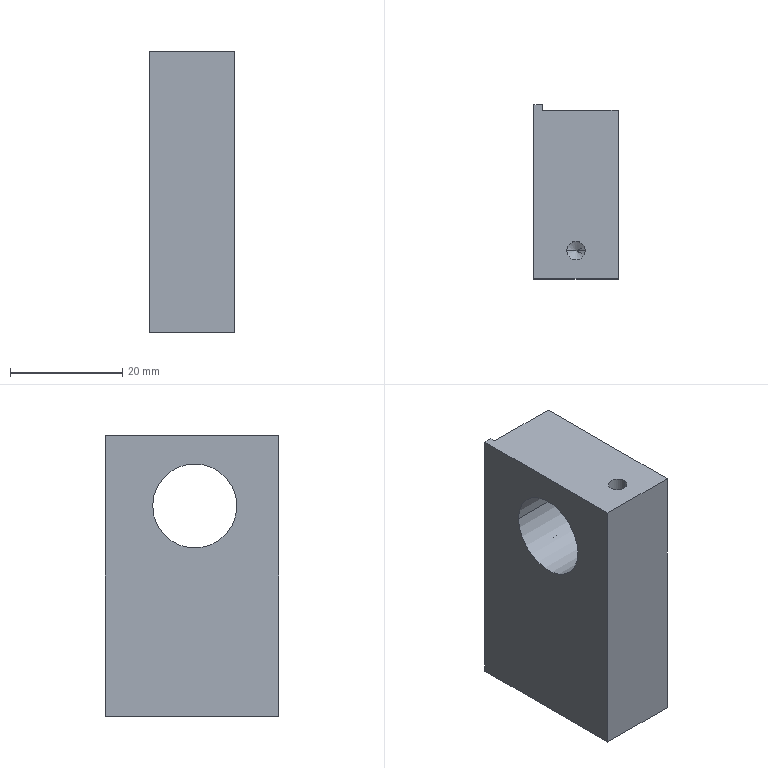Part | STEP file | 11-FG-B01011 | 1 solid | 34 faces | box 15 x 31 x 50 mm | volume 19389 mm3 | cylinder 14 | cone 12 | plane 8 | commonest cylinder face diameters 3.3 x12 15 x2
STEP:
#1=CARTESIAN_POINT('',(5.85,5.,39.9));
#2=VERTEX_POINT('',#1);
#3=CARTESIAN_POINT('',(9.15,5.,39.9));
#4=VERTEX_POINT('',#3);
#5=CARTESIAN_POINT('',(7.5,5.,39.9));
#6=DIRECTION('',(0.,0.,1.));
#7=DIRECTION('',(1.,0.,0.));
#8=AXIS2_PLACEMENT_3D('',#5,#6,#7);
#9=CIRCLE('',#8,1.65);
#10=EDGE_CURVE('',#2,#4,#9,.T.);
#11=ORIENTED_EDGE('',*,*,#10,.F.);
#12=CARTESIAN_POINT('',(5.85,5.,50.));
#13=VERTEX_POINT('',#12);
#14=CARTESIAN_POINT('',(5.85,5.,50.));
#15=DIRECTION('',(0.,0.,1.));
#16=VECTOR('',#15,1000.);
#17=LINE('',#14,#16);
#18=EDGE_CURVE('',#2,#13,#17,.T.);
#19=ORIENTED_EDGE('',*,*,#18,.T.);
#20=CARTESIAN_POINT('',(9.15,5.,50.));
#21=VERTEX_POINT('',#20);
#22=CARTESIAN_POINT('',(7.5,5.,50.));
#23=DIRECTION('',(0.,0.,1.));
#24=DIRECTION('',(1.,0.,0.));
#25=AXIS2_PLACEMENT_3D('',#22,#23,#24);
#26=CIRCLE('',#25,1.65);
#27=EDGE_CURVE('',#13,#21,#26,.T.);
#28=ORIENTED_EDGE('',*,*,#27,.T.);
#29=CARTESIAN_POINT('',(9.15,5.,50.));
#30=DIRECTION('',(0.,0.,1.));
#31=VECTOR('',#30,1000.);
#32=LINE('',#29,#31);
#33=EDGE_CURVE('',#4,#21,#32,.T.);
#34=ORIENTED_EDGE('',*,*,#33,.F.);
#35=EDGE_LOOP('',(#11,#19,#28,#34));
#36=FACE_OUTER_BOUND('',#35,.T.);
#37=CARTESIAN_POINT('',(7.5,5.,50.));
#38=DIRECTION('',(0.,0.,1.));
#39=DIRECTION('',(1.,0.,0.));
#40=AXIS2_PLACEMENT_3D('',#37,#38,#39);
#41=CYLINDRICAL_SURFACE('',#40,1.65);
#42=ADVANCED_FACE('',(#36),#41,.F.);
#43=CARTESIAN_POINT('',(7.5,5.,38.909));
#44=VERTEX_POINT('',#43);
#45=CARTESIAN_POINT('',(9.15,5.,39.9));
#46=DIRECTION('',(0.8572,0.,0.515));
#47=VECTOR('',#46,1000.);
#48=LINE('',#45,#47);
#49=EDGE_CURVE('',#44,#4,#48,.T.);
#50=ORIENTED_EDGE('',*,*,#49,.F.);
#51=CARTESIAN_POINT('',(5.85,5.,39.9));
#52=DIRECTION('',(-0.8572,0.,0.515));
#53=VECTOR('',#52,1000.);
#54=LINE('',#51,#53);
#55=EDGE_CURVE('',#44,#2,#54,.T.);
#56=ORIENTED_EDGE('',*,*,#55,.T.);
#57=ORIENTED_EDGE('',*,*,#10,.T.);
#58=EDGE_LOOP('',(#50,#56,#57));
#59=FACE_OUTER_BOUND('',#58,.T.);
#60=CARTESIAN_POINT('',(7.5,5.,39.9));
#61=DIRECTION('',(0.,0.,1.));
#62=DIRECTION('',(1.,0.,0.));
#63=AXIS2_PLACEMENT_3D('',#60,#61,#62);
#64=CONICAL_SURFACE('',#63,1.65,1.03);
#65=ADVANCED_FACE('',(#59),#64,.F.);
#66=CARTESIAN_POINT('',(6.5,19.9,43.35));
#67=VERTEX_POINT('',#66);
#68=CARTESIAN_POINT('',(6.5,19.9,46.65));
#69=VERTEX_POINT('',#68);
#70=CARTESIAN_POINT('',(6.5,19.9,45.));
#71=DIRECTION('',(0.,1.,0.));
#72=DIRECTION('',(0.,0.,1.));
#73=AXIS2_PLACEMENT_3D('',#70,#71,#72);
#74=CIRCLE('',#73,1.65);
#75=EDGE_CURVE('',#67,#69,#74,.T.);
#76=ORIENTED_EDGE('',*,*,#75,.F.);
#77=CARTESIAN_POINT('',(6.5,30.,43.35));
#78=VERTEX_POINT('',#77);
#79=CARTESIAN_POINT('',(6.5,30.,43.35));
#80=DIRECTION('',(0.,1.,0.));
#81=VECTOR('',#80,1000.);
#82=LINE('',#79,#81);
#83=EDGE_CURVE('',#67,#78,#82,.T.);
#84=ORIENTED_EDGE('',*,*,#83,.T.);
#85=CARTESIAN_POINT('',(6.5,30.,46.65));
#86=VERTEX_POINT('',#85);
#87=CARTESIAN_POINT('',(6.5,30.,45.));
#88=DIRECTION('',(0.,1.,0.));
#89=DIRECTION('',(0.,0.,1.));
#90=AXIS2_PLACEMENT_3D('',#87,#88,#89);
#91=CIRCLE('',#90,1.65);
#92=EDGE_CURVE('',#78,#86,#91,.T.);
#93=ORIENTED_EDGE('',*,*,#92,.T.);
#94=CARTESIAN_POINT('',(6.5,30.,46.65));
#95=DIRECTION('',(0.,1.,0.));
#96=VECTOR('',#95,1000.);
#97=LINE('',#94,#96);
#98=EDGE_CURVE('',#69,#86,#97,.T.);
#99=ORIENTED_EDGE('',*,*,#98,.F.);
#100=EDGE_LOOP('',(#76,#84,#93,#99));
#101=FACE_OUTER_BOUND('',#100,.T.);
#102=CARTESIAN_POINT('',(6.5,30.,45.));
#103=DIRECTION('',(0.,1.,0.));
#104=DIRECTION('',(0.,0.,1.));
#105=AXIS2_PLACEMENT_3D('',#102,#103,#104);
#106=CYLINDRICAL_SURFACE('',#105,1.65);
#107=ADVANCED_FACE('',(#101),#106,.F.);
#108=CARTESIAN_POINT('',(6.5,18.909,45.));
#109=VERTEX_POINT('',#108);
#110=CARTESIAN_POINT('',(6.5,19.9,46.65));
#111=DIRECTION('',(0.,0.515,0.8572));
#112=VECTOR('',#111,1000.);
#113=LINE('',#110,#112);
#114=EDGE_CURVE('',#109,#69,#113,.T.);
#115=ORIENTED_EDGE('',*,*,#114,.F.);
#116=CARTESIAN_POINT('',(6.5,19.9,43.35));
#117=DIRECTION('',(0.,0.515,-0.8572));
#118=VECTOR('',#117,1000.);
#119=LINE('',#116,#118);
#120=EDGE_CURVE('',#109,#67,#119,.T.);
#121=ORIENTED_EDGE('',*,*,#120,.T.);
#122=ORIENTED_EDGE('',*,*,#75,.T.);
#123=EDGE_LOOP('',(#115,#121,#122));
#124=FACE_OUTER_BOUND('',#123,.T.);
#125=CARTESIAN_POINT('',(6.5,19.9,45.));
#126=DIRECTION('',(0.,1.,0.));
#127=DIRECTION('',(0.,0.,1.));
#128=AXIS2_PLACEMENT_3D('',#125,#126,#127);
#129=CONICAL_SURFACE('',#128,1.65,1.03);
#130=ADVANCED_FACE('',(#124),#129,.F.);
#131=CARTESIAN_POINT('',(6.5,19.9,28.35));
#132=VERTEX_POINT('',#131);
#133=CARTESIAN_POINT('',(6.5,19.9,31.65));
#134=VERTEX_POINT('',#133);
#135=CARTESIAN_POINT('',(6.5,19.9,30.));
#136=DIRECTION('',(0.,1.,0.));
#137=DIRECTION('',(0.,0.,1.));
#138=AXIS2_PLACEMENT_3D('',#135,#136,#137);
#139=CIRCLE('',#138,1.65);
#140=EDGE_CURVE('',#132,#134,#139,.T.);
#141=ORIENTED_EDGE('',*,*,#140,.F.);
#142=CARTESIAN_POINT('',(6.5,30.,28.35));
#143=VERTEX_POINT('',#142);
#144=CARTESIAN_POINT('',(6.5,30.,28.35));
#145=DIRECTION('',(0.,1.,0.));
#146=VECTOR('',#145,1000.);
#147=LINE('',#144,#146);
#148=EDGE_CURVE('',#132,#143,#147,.T.);
#149=ORIENTED_EDGE('',*,*,#148,.T.);
#150=CARTESIAN_POINT('',(6.5,30.,31.65));
#151=VERTEX_POINT('',#150);
#152=CARTESIAN_POINT('',(6.5,30.,30.));
#153=DIRECTION('',(0.,1.,0.));
#154=DIRECTION('',(0.,0.,1.));
#155=AXIS2_PLACEMENT_3D('',#152,#153,#154);
#156=CIRCLE('',#155,1.65);
#157=EDGE_CURVE('',#143,#151,#156,.T.);
#158=ORIENTED_EDGE('',*,*,#157,.T.);
#159=CARTESIAN_POINT('',(6.5,30.,31.65));
#160=DIRECTION('',(0.,1.,0.));
#161=VECTOR('',#160,1000.);
#162=LINE('',#159,#161);
#163=EDGE_CURVE('',#134,#151,#162,.T.);
#164=ORIENTED_EDGE('',*,*,#163,.F.);
#165=EDGE_LOOP('',(#141,#149,#158,#164));
#166=FACE_OUTER_BOUND('',#165,.T.);
#167=CARTESIAN_POINT('',(6.5,30.,30.));
#168=DIRECTION('',(0.,1.,0.));
#169=DIRECTION('',(0.,0.,1.));
#170=AXIS2_PLACEMENT_3D('',#167,#168,#169);
#171=CYLINDRICAL_SURFACE('',#170,1.65);
#172=ADVANCED_FACE('',(#166),#171,.F.);
#173=CARTESIAN_POINT('',(6.5,18.909,30.));
#174=VERTEX_POINT('',#173);
#175=CARTESIAN_POINT('',(6.5,19.9,31.65));
#176=DIRECTION('',(0.,0.515,0.8572));
#177=VECTOR('',#176,1000.);
#178=LINE('',#175,#177);
#179=EDGE_CURVE('',#174,#134,#178,.T.);
#180=ORIENTED_EDGE('',*,*,#179,.F.);
#181=CARTESIAN_POINT('',(6.5,19.9,28.35));
#182=DIRECTION('',(0.,0.515,-0.8572));
#183=VECTOR('',#182,1000.);
#184=LINE('',#181,#183);
#185=EDGE_CURVE('',#174,#132,#184,.T.);
#186=ORIENTED_EDGE('',*,*,#185,.T.);
#187=ORIENTED_EDGE('',*,*,#140,.T.);
#188=EDGE_LOOP('',(#180,#186,#187));
#189=FACE_OUTER_BOUND('',#188,.T.);
#190=CARTESIAN_POINT('',(6.5,19.9,30.));
#191=DIRECTION('',(0.,1.,0.));
#192=DIRECTION('',(0.,0.,1.));
#193=AXIS2_PLACEMENT_3D('',#190,#191,#192);
#194=CONICAL_SURFACE('',#193,1.65,1.03);
#195=ADVANCED_FACE('',(#189),#194,.F.);
#196=CARTESIAN_POINT('',(9.15,5.,10.1));
#197=VERTEX_POINT('',#196);
#198=CARTESIAN_POINT('',(5.85,5.,10.1));
#199=VERTEX_POINT('',#198);
#200=CARTESIAN_POINT('',(7.5,5.,10.1));
#201=DIRECTION('',(0.,0.,-1.));
#202=DIRECTION('',(-1.,0.,0.));
#203=AXIS2_PLACEMENT_3D('',#200,#201,#202);
#204=CIRCLE('',#203,1.65);
#205=EDGE_CURVE('',#197,#199,#204,.T.);
#206=ORIENTED_EDGE('',*,*,#205,.F.);
#207=CARTESIAN_POINT('',(9.15,5.,0.));
#208=VERTEX_POINT('',#207);
#209=CARTESIAN_POINT('',(9.15,5.,0.));
#210=DIRECTION('',(0.,0.,-1.));
#211=VECTOR('',#210,1000.);
#212=LINE('',#209,#211);
#213=EDGE_CURVE('',#197,#208,#212,.T.);
#214=ORIENTED_EDGE('',*,*,#213,.T.);
#215=CARTESIAN_POINT('',(5.85,5.,0.));
#216=VERTEX_POINT('',#215);
#217=CARTESIAN_POINT('',(7.5,5.,0.));
#218=DIRECTION('',(0.,0.,-1.));
#219=DIRECTION('',(-1.,0.,0.));
#220=AXIS2_PLACEMENT_3D('',#217,#218,#219);
#221=CIRCLE('',#220,1.65);
#222=EDGE_CURVE('',#208,#216,#221,.T.);
#223=ORIENTED_EDGE('',*,*,#222,.T.);
#224=CARTESIAN_POINT('',(5.85,5.,0.));
#225=DIRECTION('',(0.,0.,-1.));
#226=VECTOR('',#225,1000.);
#227=LINE('',#224,#226);
#228=EDGE_CURVE('',#199,#216,#227,.T.);
#229=ORIENTED_EDGE('',*,*,#228,.F.);
#230=EDGE_LOOP('',(#206,#214,#223,#229));
#231=FACE_OUTER_BOUND('',#230,.T.);
#232=CARTESIAN_POINT('',(7.5,5.,0.));
#233=DIRECTION('',(0.,0.,-1.));
#234=DIRECTION('',(-1.,0.,0.));
#235=AXIS2_PLACEMENT_3D('',#232,#233,#234);
#236=CYLINDRICAL_SURFACE('',#235,1.65);
#237=ADVANCED_FACE('',(#231),#236,.F.);
#238=CARTESIAN_POINT('',(7.5,5.,11.091));
#239=VERTEX_POINT('',#238);
#240=CARTESIAN_POINT('',(5.85,5.,10.1));
#241=DIRECTION('',(-0.8572,0.,-0.515));
#242=VECTOR('',#241,1000.);
#243=LINE('',#240,#242);
#244=EDGE_CURVE('',#239,#199,#243,.T.);
#245=ORIENTED_EDGE('',*,*,#244,.F.);
#246=CARTESIAN_POINT('',(9.15,5.,10.1));
#247=DIRECTION('',(0.8572,0.,-0.515));
#248=VECTOR('',#247,1000.);
#249=LINE('',#246,#248);
#250=EDGE_CURVE('',#239,#197,#249,.T.);
#251=ORIENTED_EDGE('',*,*,#250,.T.);
#252=ORIENTED_EDGE('',*,*,#205,.T.);
#253=EDGE_LOOP('',(#245,#251,#252));
#254=FACE_OUTER_BOUND('',#253,.T.);
#255=CARTESIAN_POINT('',(7.5,5.,10.1));
#256=DIRECTION('',(0.,0.,-1.));
#257=DIRECTION('',(-1.,0.,0.));
#258=AXIS2_PLACEMENT_3D('',#255,#256,#257);
#259=CONICAL_SURFACE('',#258,1.65,1.03);
#260=ADVANCED_FACE('',(#254),#259,.F.);
#261=CARTESIAN_POINT('',(6.5,19.9,3.35));
#262=VERTEX_POINT('',#261);
#263=CARTESIAN_POINT('',(6.5,19.9,6.65));
#264=VERTEX_POINT('',#263);
#265=CARTESIAN_POINT('',(6.5,19.9,5.));
#266=DIRECTION('',(0.,1.,0.));
#267=DIRECTION('',(0.,0.,1.));
#268=AXIS2_PLACEMENT_3D('',#265,#266,#267);
#269=CIRCLE('',#268,1.65);
#270=EDGE_CURVE('',#262,#264,#269,.T.);
#271=ORIENTED_EDGE('',*,*,#270,.F.);
#272=CARTESIAN_POINT('',(6.5,30.,3.35));
#273=VERTEX_POINT('',#272);
#274=CARTESIAN_POINT('',(6.5,30.,3.35));
#275=DIRECTION('',(0.,1.,0.));
#276=VECTOR('',#275,1000.);
#277=LINE('',#274,#276);
#278=EDGE_CURVE('',#262,#273,#277,.T.);
#279=ORIENTED_EDGE('',*,*,#278,.T.);
#280=CARTESIAN_POINT('',(6.5,30.,6.65));
#281=VERTEX_POINT('',#280);
#282=CARTESIAN_POINT('',(6.5,30.,5.));
#283=DIRECTION('',(0.,1.,0.));
#284=DIRECTION('',(0.,0.,1.));
#285=AXIS2_PLACEMENT_3D('',#282,#283,#284);
#286=CIRCLE('',#285,1.65);
#287=EDGE_CURVE('',#273,#281,#286,.T.);
#288=ORIENTED_EDGE('',*,*,#287,.T.);
#289=CARTESIAN_POINT('',(6.5,30.,6.65));
#290=DIRECTION('',(0.,1.,0.));
#291=VECTOR('',#290,1000.);
#292=LINE('',#289,#291);
#293=EDGE_CURVE('',#264,#281,#292,.T.);
#294=ORIENTED_EDGE('',*,*,#293,.F.);
#295=EDGE_LOOP('',(#271,#279,#288,#294));
#296=FACE_OUTER_BOUND('',#295,.T.);
#297=CARTESIAN_POINT('',(6.5,30.,5.));
#298=DIRECTION('',(0.,1.,0.));
#299=DIRECTION('',(0.,0.,1.));
#300=AXIS2_PLACEMENT_3D('',#297,#298,#299);
#301=CYLINDRICAL_SURFACE('',#300,1.65);
#302=ADVANCED_FACE('',(#296),#301,.F.);
#303=CARTESIAN_POINT('',(6.5,18.909,5.));
#304=VERTEX_POINT('',#303);
#305=CARTESIAN_POINT('',(6.5,19.9,6.65));
#306=DIRECTION('',(0.,0.515,0.8572));
#307=VECTOR('',#306,1000.);
#308=LINE('',#305,#307);
#309=EDGE_CURVE('',#304,#264,#308,.T.);
#310=ORIENTED_EDGE('',*,*,#309,.F.);
#311=CARTESIAN_POINT('',(6.5,19.9,3.35));
#312=DIRECTION('',(0.,0.515,-0.8572));
#313=VECTOR('',#312,1000.);
#314=LINE('',#311,#313);
#315=EDGE_CURVE('',#304,#262,#314,.T.);
#316=ORIENTED_EDGE('',*,*,#315,.T.);
#317=ORIENTED_EDGE('',*,*,#270,.T.);
#318=EDGE_LOOP('',(#310,#316,#317));
#319=FACE_OUTER_BOUND('',#318,.T.);
#320=CARTESIAN_POINT('',(6.5,19.9,5.));
#321=DIRECTION('',(0.,1.,0.));
#322=DIRECTION('',(0.,0.,1.));
#323=AXIS2_PLACEMENT_3D('',#320,#321,#322);
#324=CONICAL_SURFACE('',#323,1.65,1.03);
#325=ADVANCED_FACE('',(#319),#324,.F.);
#326=CARTESIAN_POINT('',(6.5,19.9,18.35));
#327=VERTEX_POINT('',#326);
#328=CARTESIAN_POINT('',(6.5,19.9,21.65));
#329=VERTEX_POINT('',#328);
#330=CARTESIAN_POINT('',(6.5,19.9,20.));
#331=DIRECTION('',(0.,1.,0.));
#332=DIRECTION('',(0.,0.,1.));
#333=AXIS2_PLACEMENT_3D('',#330,#331,#332);
#334=CIRCLE('',#333,1.65);
#335=EDGE_CURVE('',#327,#329,#334,.T.);
#336=ORIENTED_EDGE('',*,*,#335,.F.);
#337=CARTESIAN_POINT('',(6.5,30.,18.35));
#338=VERTEX_POINT('',#337);
#339=CARTESIAN_POINT('',(6.5,30.,18.35));
#340=DIRECTION('',(0.,1.,0.));
#341=VECTOR('',#340,1000.);
#342=LINE('',#339,#341);
#343=EDGE_CURVE('',#327,#338,#342,.T.);
#344=ORIENTED_EDGE('',*,*,#343,.T.);
#345=CARTESIAN_POINT('',(6.5,30.,21.65));
#346=VERTEX_POINT('',#345);
#347=CARTESIAN_POINT('',(6.5,30.,20.));
#348=DIRECTION('',(0.,1.,0.));
#349=DIRECTION('',(0.,0.,1.));
#350=AXIS2_PLACEMENT_3D('',#347,#348,#349);
#351=CIRCLE('',#350,1.65);
#352=EDGE_CURVE('',#338,#346,#351,.T.);
#353=ORIENTED_EDGE('',*,*,#352,.T.);
#354=CARTESIAN_POINT('',(6.5,30.,21.65));
#355=DIRECTION('',(0.,1.,0.));
#356=VECTOR('',#355,1000.);
#357=LINE('',#354,#356);
#358=EDGE_CURVE('',#329,#346,#357,.T.);
#359=ORIENTED_EDGE('',*,*,#358,.F.);
#360=EDGE_LOOP('',(#336,#344,#353,#359));
#361=FACE_OUTER_BOUND('',#360,.T.);
#362=CARTESIAN_POINT('',(6.5,30.,20.));
#363=DIRECTION('',(0.,1.,0.));
#364=DIRECTION('',(0.,0.,1.));
#365=AXIS2_PLACEMENT_3D('',#362,#363,#364);
#366=CYLINDRICAL_SURFACE('',#365,1.65);
#367=ADVANCED_FACE('',(#361),#366,.F.);
#368=CARTESIAN_POINT('',(6.5,18.909,20.));
#369=VERTEX_POINT('',#368);
#370=CARTESIAN_POINT('',(6.5,19.9,21.65));
#371=DIRECTION('',(0.,0.515,0.8572));
#372=VECTOR('',#371,1000.);
#373=LINE('',#370,#372);
#374=EDGE_CURVE('',#369,#329,#373,.T.);
#375=ORIENTED_EDGE('',*,*,#374,.F.);
#376=CARTESIAN_POINT('',(6.5,19.9,18.35));
#377=DIRECTION('',(0.,0.515,-0.8572));
#378=VECTOR('',#377,1000.);
#379=LINE('',#376,#378);
#380=EDGE_CURVE('',#369,#327,#379,.T.);
#381=ORIENTED_EDGE('',*,*,#380,.T.);
#382=ORIENTED_EDGE('',*,*,#335,.T.);
#383=EDGE_LOOP('',(#375,#381,#382));
#384=FACE_OUTER_BOUND('',#383,.T.);
#385=CARTESIAN_POINT('',(6.5,19.9,20.));
#386=DIRECTION('',(0.,1.,0.));
#387=DIRECTION('',(0.,0.,1.));
#388=AXIS2_PLACEMENT_3D('',#385,#386,#387);
#389=CONICAL_SURFACE('',#388,1.65,1.03);
#390=ADVANCED_FACE('',(#384),#389,.F.);
#391=CARTESIAN_POINT('',(15.,22.5,37.5));
#392=VERTEX_POINT('',#391);
#393=CARTESIAN_POINT('',(15.,7.5,37.5));
#394=VERTEX_POINT('',#393);
#395=CARTESIAN_POINT('',(15.,15.,37.5));
#396=DIRECTION('',(-1.,0.,0.));
#397=DIRECTION('',(0.,-1.,0.));
#398=AXIS2_PLACEMENT_3D('',#395,#396,#397);
#399=CIRCLE('',#398,7.5);
#400=EDGE_CURVE('',#392,#394,#399,.T.);
#401=ORIENTED_EDGE('',*,*,#400,.F.);
#402=CARTESIAN_POINT('',(0.,22.5,37.5));
#403=VERTEX_POINT('',#402);
#404=CARTESIAN_POINT('',(15.,22.5,37.5));
#405=DIRECTION('',(-1.,0.,0.));
#406=VECTOR('',#405,1000.);
#407=LINE('',#404,#406);
#408=EDGE_CURVE('',#392,#403,#407,.T.);
#409=ORIENTED_EDGE('',*,*,#408,.T.);
#410=CARTESIAN_POINT('',(0.,7.5,37.5));
#411=VERTEX_POINT('',#410);
#412=CARTESIAN_POINT('',(0.,15.,37.5));
#413=DIRECTION('',(-1.,0.,0.));
#414=DIRECTION('',(0.,-1.,0.));
#415=AXIS2_PLACEMENT_3D('',#412,#413,#414);
#416=CIRCLE('',#415,7.5);
#417=EDGE_CURVE('',#403,#411,#416,.T.);
#418=ORIENTED_EDGE('',*,*,#417,.T.);
#419=CARTESIAN_POINT('',(15.,7.5,37.5));
#420=DIRECTION('',(-1.,0.,0.));
#421=VECTOR('',#420,1000.);
#422=LINE('',#419,#421);
#423=EDGE_CURVE('',#394,#411,#422,.T.);
#424=ORIENTED_EDGE('',*,*,#423,.F.);
#425=EDGE_LOOP('',(#401,#409,#418,#424));
#426=FACE_OUTER_BOUND('',#425,.T.);
#427=CARTESIAN_POINT('',(15.,15.,37.5));
#428=DIRECTION('',(-1.,0.,0.));
#429=DIRECTION('',(0.,-1.,0.));
#430=AXIS2_PLACEMENT_3D('',#427,#428,#429);
#431=CYLINDRICAL_SURFACE('',#430,7.5);
#432=ADVANCED_FACE('',(#426),#431,.F.);
#433=CARTESIAN_POINT('',(6.5,30.,45.));
#434=DIRECTION('',(0.,1.,0.));
#435=DIRECTION('',(0.,0.,1.));
#436=AXIS2_PLACEMENT_3D('',#433,#434,#435);
#437=CIRCLE('',#436,1.65);
#438=EDGE_CURVE('',#86,#78,#437,.T.);
#439=ORIENTED_EDGE('',*,*,#438,.F.);
#440=ORIENTED_EDGE('',*,*,#92,.F.);
#441=EDGE_LOOP('',(#439,#440));
#442=FACE_BOUND('',#441,.T.);
#443=CARTESIAN_POINT('',(6.5,30.,30.));
#444=DIRECTION('',(0.,1.,0.));
#445=DIRECTION('',(0.,0.,1.));
#446=AXIS2_PLACEMENT_3D('',#443,#444,#445);
#447=CIRCLE('',#446,1.65);
#448=EDGE_CURVE('',#151,#143,#447,.T.);
#449=ORIENTED_EDGE('',*,*,#448,.F.);
#450=ORIENTED_EDGE('',*,*,#157,.F.);
#451=EDGE_LOOP('',(#449,#450));
#452=FACE_BOUND('',#451,.T.);
#453=CARTESIAN_POINT('',(6.5,30.,20.));
#454=DIRECTION('',(0.,1.,0.));
#455=DIRECTION('',(0.,0.,1.));
#456=AXIS2_PLACEMENT_3D('',#453,#454,#455);
#457=CIRCLE('',#456,1.65);
#458=EDGE_CURVE('',#346,#338,#457,.T.);
#459=ORIENTED_EDGE('',*,*,#458,.F.);
#460=ORIENTED_EDGE('',*,*,#352,.F.);
#461=EDGE_LOOP('',(#459,#460));
#462=FACE_BOUND('',#461,.T.);
#463=CARTESIAN_POINT('',(6.5,30.,5.));
#464=DIRECTION('',(0.,1.,0.));
#465=DIRECTION('',(0.,0.,1.));
#466=AXIS2_PLACEMENT_3D('',#463,#464,#465);
#467=CIRCLE('',#466,1.65);
#468=EDGE_CURVE('',#281,#273,#467,.T.);
#469=ORIENTED_EDGE('',*,*,#468,.F.);
#470=ORIENTED_EDGE('',*,*,#287,.F.);
#471=EDGE_LOOP('',(#469,#470));
#472=FACE_BOUND('',#471,.T.);
#473=CARTESIAN_POINT('',(1.5,30.,50.));
#474=VERTEX_POINT('',#473);
#475=CARTESIAN_POINT('',(1.5,30.,0.));
#476=VERTEX_POINT('',#475);
#477=CARTESIAN_POINT('',(1.5,30.,0.));
#478=DIRECTION('',(0.,0.,-1.));
#479=VECTOR('',#478,1000.);
#480=LINE('',#477,#479);
#481=EDGE_CURVE('',#474,#476,#480,.T.);
#482=ORIENTED_EDGE('',*,*,#481,.F.);
#483=CARTESIAN_POINT('',(15.,30.,50.));
#484=VERTEX_POINT('',#483);
#485=CARTESIAN_POINT('',(0.,30.,50.));
#486=DIRECTION('',(-1.,0.,0.));
#487=VECTOR('',#486,1000.);
#488=LINE('',#485,#487);
#489=EDGE_CURVE('',#484,#474,#488,.T.);
#490=ORIENTED_EDGE('',*,*,#489,.F.);
#491=CARTESIAN_POINT('',(15.,30.,0.));
#492=VERTEX_POINT('',#491);
#493=CARTESIAN_POINT('',(15.,30.,50.));
#494=DIRECTION('',(0.,0.,-1.));
#495=VECTOR('',#494,1000.);
#496=LINE('',#493,#495);
#497=EDGE_CURVE('',#484,#492,#496,.T.);
#498=ORIENTED_EDGE('',*,*,#497,.T.);
#499=CARTESIAN_POINT('',(0.,30.,0.));
#500=DIRECTION('',(-1.,0.,0.));
#501=VECTOR('',#500,1000.);
#502=LINE('',#499,#501);
#503=EDGE_CURVE('',#492,#476,#502,.T.);
#504=ORIENTED_EDGE('',*,*,#503,.T.);
#505=EDGE_LOOP('',(#482,#490,#498,#504));
#506=FACE_OUTER_BOUND('',#505,.T.);
#507=CARTESIAN_POINT('',(0.,30.,50.));
#508=DIRECTION('',(0.,-1.,0.));
#509=DIRECTION('',(0.,0.,-1.));
#510=AXIS2_PLACEMENT_3D('',#507,#508,#509);
#511=PLANE('',#510);
#512=ADVANCED_FACE('',(#442,#452,#462,#472,#506),#511,.F.);
#513=CARTESIAN_POINT('',(0.,15.,37.5));
#514=DIRECTION('',(-1.,0.,0.));
#515=DIRECTION('',(0.,-1.,0.));
#516=AXIS2_PLACEMENT_3D('',#513,#514,#515);
#517=CIRCLE('',#516,7.5);
#518=EDGE_CURVE('',#411,#403,#517,.T.);
#519=ORIENTED_EDGE('',*,*,#518,.F.);
#520=ORIENTED_EDGE('',*,*,#417,.F.);
#521=EDGE_LOOP('',(#519,#520));
#522=FACE_BOUND('',#521,.T.);
#523=CARTESIAN_POINT('',(0.,31.,0.));
#524=VERTEX_POINT('',#523);
#525=CARTESIAN_POINT('',(0.,0.,0.));
#526=VERTEX_POINT('',#525);
#527=CARTESIAN_POINT('',(0.,0.,0.));
#528=DIRECTION('',(0.,-1.,0.));
#529=VECTOR('',#528,1000.);
#530=LINE('',#527,#529);
#531=EDGE_CURVE('',#524,#526,#530,.T.);
#532=ORIENTED_EDGE('',*,*,#531,.T.);
#533=CARTESIAN_POINT('',(0.,0.,50.));
#534=VERTEX_POINT('',#533);
#535=CARTESIAN_POINT('',(0.,0.,50.));
#536=DIRECTION('',(0.,0.,-1.));
#537=VECTOR('',#536,1000.);
#538=LINE('',#535,#537);
#539=EDGE_CURVE('',#534,#526,#538,.T.);
#540=ORIENTED_EDGE('',*,*,#539,.F.);
#541=CARTESIAN_POINT('',(0.,31.,50.));
#542=VERTEX_POINT('',#541);
#543=CARTESIAN_POINT('',(0.,0.,50.));
#544=DIRECTION('',(0.,-1.,0.));
#545=VECTOR('',#544,1000.);
#546=LINE('',#543,#545);
#547=EDGE_CURVE('',#542,#534,#546,.T.);
#548=ORIENTED_EDGE('',*,*,#547,.F.);
#549=CARTESIAN_POINT('',(0.,31.,0.));
#550=DIRECTION('',(0.,0.,1.));
#551=VECTOR('',#550,1000.);
#552=LINE('',#549,#551);
#553=EDGE_CURVE('',#524,#542,#552,.T.);
#554=ORIENTED_EDGE('',*,*,#553,.F.);
#555=EDGE_LOOP('',(#532,#540,#548,#554));
#556=FACE_OUTER_BOUND('',#555,.T.);
#557=CARTESIAN_POINT('',(0.,0.,50.));
#558=DIRECTION('',(1.,0.,0.));
#559=DIRECTION('',(0.,1.,0.));
#560=AXIS2_PLACEMENT_3D('',#557,#558,#559);
#561=PLANE('',#560);
#562=ADVANCED_FACE('',(#522,#556),#561,.F.);
#563=CARTESIAN_POINT('',(15.,0.,0.));
#564=VERTEX_POINT('',#563);
#565=CARTESIAN_POINT('',(0.,0.,0.));
#566=DIRECTION('',(1.,0.,0.));
#567=VECTOR('',#566,1000.);
#568=LINE('',#565,#567);
#569=EDGE_CURVE('',#526,#564,#568,.T.);
#570=ORIENTED_EDGE('',*,*,#569,.T.);
#571=CARTESIAN_POINT('',(15.,0.,50.));
#572=VERTEX_POINT('',#571);
#573=CARTESIAN_POINT('',(15.,0.,50.));
#574=DIRECTION('',(0.,0.,-1.));
#575=VECTOR('',#574,1000.);
#576=LINE('',#573,#575);
#577=EDGE_CURVE('',#572,#564,#576,.T.);
#578=ORIENTED_EDGE('',*,*,#577,.F.);
#579=CARTESIAN_POINT('',(0.,0.,50.));
#580=DIRECTION('',(1.,0.,0.));
#581=VECTOR('',#580,1000.);
#582=LINE('',#579,#581);
#583=EDGE_CURVE('',#534,#572,#582,.T.);
#584=ORIENTED_EDGE('',*,*,#583,.F.);
#585=ORIENTED_EDGE('',*,*,#539,.T.);
#586=EDGE_LOOP('',(#570,#578,#584,#585));
#587=FACE_OUTER_BOUND('',#586,.T.);
#588=CARTESIAN_POINT('',(0.,0.,50.));
#589=DIRECTION('',(0.,1.,0.));
#590=DIRECTION('',(0.,0.,1.));
#591=AXIS2_PLACEMENT_3D('',#588,#589,#590);
#592=PLANE('',#591);
#593=ADVANCED_FACE('',(#587),#592,.F.);
#594=CARTESIAN_POINT('',(15.,15.,37.5));
#595=DIRECTION('',(-1.,0.,0.));
#596=DIRECTION('',(0.,-1.,0.));
#597=AXIS2_PLACEMENT_3D('',#594,#595,#596);
#598=CIRCLE('',#597,7.5);
#599=EDGE_CURVE('',#394,#392,#598,.T.);
#600=ORIENTED_EDGE('',*,*,#599,.T.);
#601=ORIENTED_EDGE('',*,*,#400,.T.);
#602=EDGE_LOOP('',(#600,#601));
#603=FACE_BOUND('',#602,.T.);
#604=CARTESIAN_POINT('',(15.,0.,0.));
#605=DIRECTION('',(0.,1.,0.));
#606=VECTOR('',#605,1000.);
#607=LINE('',#604,#606);
#608=EDGE_CURVE('',#564,#492,#607,.T.);
#609=ORIENTED_EDGE('',*,*,#608,.T.);
#610=ORIENTED_EDGE('',*,*,#497,.F.);
#611=CARTESIAN_POINT('',(15.,0.,50.));
#612=DIRECTION('',(0.,1.,0.));
#613=VECTOR('',#612,1000.);
#614=LINE('',#611,#613);
#615=EDGE_CURVE('',#572,#484,#614,.T.);
#616=ORIENTED_EDGE('',*,*,#615,.F.);
#617=ORIENTED_EDGE('',*,*,#577,.T.);
#618=EDGE_LOOP('',(#609,#610,#616,#617));
#619=FACE_OUTER_BOUND('',#618,.T.);
#620=CARTESIAN_POINT('',(15.,0.,50.));
#621=DIRECTION('',(-1.,0.,0.));
#622=DIRECTION('',(0.,-1.,0.));
#623=AXIS2_PLACEMENT_3D('',#620,#621,#622);
#624=PLANE('',#623);
#625=ADVANCED_FACE('',(#603,#619),#624,.F.);
#626=CARTESIAN_POINT('',(7.5,5.,50.));
#627=DIRECTION('',(0.,0.,1.));
#628=DIRECTION('',(1.,0.,0.));
#629=AXIS2_PLACEMENT_3D('',#626,#627,#628);
#630=CIRCLE('',#629,1.65);
#631=EDGE_CURVE('',#21,#13,#630,.T.);
#632=ORIENTED_EDGE('',*,*,#631,.F.);
#633=ORIENTED_EDGE('',*,*,#27,.F.);
#634=EDGE_LOOP('',(#632,#633));
#635=FACE_BOUND('',#634,.T.);
#636=ORIENTED_EDGE('',*,*,#547,.T.);
#637=ORIENTED_EDGE('',*,*,#583,.T.);
#638=ORIENTED_EDGE('',*,*,#615,.T.);
#639=ORIENTED_EDGE('',*,*,#489,.T.);
#640=CARTESIAN_POINT('',(1.5,31.,50.));
#641=VERTEX_POINT('',#640);
#642=CARTESIAN_POINT('',(1.5,31.,50.));
#643=DIRECTION('',(0.,-1.,0.));
#644=VECTOR('',#643,1000.);
#645=LINE('',#642,#644);
#646=EDGE_CURVE('',#641,#474,#645,.T.);
#647=ORIENTED_EDGE('',*,*,#646,.F.);
#648=CARTESIAN_POINT('',(0.,31.,50.));
#649=DIRECTION('',(1.,0.,0.));
#650=VECTOR('',#649,1000.);
#651=LINE('',#648,#650);
#652=EDGE_CURVE('',#542,#641,#651,.T.);
#653=ORIENTED_EDGE('',*,*,#652,.F.);
#654=EDGE_LOOP('',(#636,#637,#638,#639,#647,#653));
#655=FACE_OUTER_BOUND('',#654,.T.);
#656=CARTESIAN_POINT('',(0.,30.,50.));
#657=DIRECTION('',(0.,0.,-1.));
#658=DIRECTION('',(-1.,0.,0.));
#659=AXIS2_PLACEMENT_3D('',#656,#657,#658);
#660=PLANE('',#659);
#661=ADVANCED_FACE('',(#635,#655),#660,.F.);
#662=CARTESIAN_POINT('',(7.5,5.,0.));
#663=DIRECTION('',(0.,0.,-1.));
#664=DIRECTION('',(-1.,0.,0.));
#665=AXIS2_PLACEMENT_3D('',#662,#663,#664);
#666=CIRCLE('',#665,1.65);
#667=EDGE_CURVE('',#216,#208,#666,.T.);
#668=ORIENTED_EDGE('',*,*,#667,.F.);
#669=ORIENTED_EDGE('',*,*,#222,.F.);
#670=EDGE_LOOP('',(#668,#669));
#671=FACE_BOUND('',#670,.T.);
#672=ORIENTED_EDGE('',*,*,#531,.F.);
#673=CARTESIAN_POINT('',(1.5,31.,0.));
#674=VERTEX_POINT('',#673);
#675=CARTESIAN_POINT('',(0.,31.,0.));
#676=DIRECTION('',(-1.,0.,0.));
#677=VECTOR('',#676,1000.);
#678=LINE('',#675,#677);
#679=EDGE_CURVE('',#674,#524,#678,.T.);
#680=ORIENTED_EDGE('',*,*,#679,.F.);
#681=CARTESIAN_POINT('',(1.5,31.,0.));
#682=DIRECTION('',(0.,-1.,0.));
#683=VECTOR('',#682,1000.);
#684=LINE('',#681,#683);
#685=EDGE_CURVE('',#674,#476,#684,.T.);
#686=ORIENTED_EDGE('',*,*,#685,.T.);
#687=ORIENTED_EDGE('',*,*,#503,.F.);
#688=ORIENTED_EDGE('',*,*,#608,.F.);
#689=ORIENTED_EDGE('',*,*,#569,.F.);
#690=EDGE_LOOP('',(#672,#680,#686,#687,#688,#689));
#691=FACE_OUTER_BOUND('',#690,.T.);
#692=CARTESIAN_POINT('',(0.,30.,0.));
#693=DIRECTION('',(0.,0.,-1.));
#694=DIRECTION('',(-1.,0.,0.));
#695=AXIS2_PLACEMENT_3D('',#692,#693,#694);
#696=PLANE('',#695);
#697=ADVANCED_FACE('',(#671,#691),#696,.T.);
#698=ORIENTED_EDGE('',*,*,#408,.F.);
#699=ORIENTED_EDGE('',*,*,#599,.F.);
#700=ORIENTED_EDGE('',*,*,#423,.T.);
#701=ORIENTED_EDGE('',*,*,#518,.T.);
#702=EDGE_LOOP('',(#698,#699,#700,#701));
#703=FACE_OUTER_BOUND('',#702,.T.);
#704=CARTESIAN_POINT('',(15.,15.,37.5));
#705=DIRECTION('',(-1.,0.,0.));
#706=DIRECTION('',(0.,-1.,0.));
#707=AXIS2_PLACEMENT_3D('',#704,#705,#706);
#708=CYLINDRICAL_SURFACE('',#707,7.5);
#709=ADVANCED_FACE('',(#703),#708,.F.);
#710=ORIENTED_EDGE('',*,*,#380,.F.);
#711=ORIENTED_EDGE('',*,*,#374,.T.);
#712=CARTESIAN_POINT('',(6.5,19.9,20.));
#713=DIRECTION('',(0.,1.,0.));
#714=DIRECTION('',(0.,0.,1.));
#715=AXIS2_PLACEMENT_3D('',#712,#713,#714);
#716=CIRCLE('',#715,1.65);
#717=EDGE_CURVE('',#329,#327,#716,.T.);
#718=ORIENTED_EDGE('',*,*,#717,.T.);
#719=EDGE_LOOP('',(#710,#711,#718));
#720=FACE_OUTER_BOUND('',#719,.T.);
#721=CARTESIAN_POINT('',(6.5,19.9,20.));
#722=DIRECTION('',(0.,1.,0.));
#723=DIRECTION('',(0.,0.,1.));
#724=AXIS2_PLACEMENT_3D('',#721,#722,#723);
#725=CONICAL_SURFACE('',#724,1.65,1.03);
#726=ADVANCED_FACE('',(#720),#725,.F.);
#727=ORIENTED_EDGE('',*,*,#343,.F.);
#728=ORIENTED_EDGE('',*,*,#717,.F.);
#729=ORIENTED_EDGE('',*,*,#358,.T.);
#730=ORIENTED_EDGE('',*,*,#458,.T.);
#731=EDGE_LOOP('',(#727,#728,#729,#730));
#732=FACE_OUTER_BOUND('',#731,.T.);
#733=CARTESIAN_POINT('',(6.5,30.,20.));
#734=DIRECTION('',(0.,1.,0.));
#735=DIRECTION('',(0.,0.,1.));
#736=AXIS2_PLACEMENT_3D('',#733,#734,#735);
#737=CYLINDRICAL_SURFACE('',#736,1.65);
#738=ADVANCED_FACE('',(#732),#737,.F.);
#739=ORIENTED_EDGE('',*,*,#315,.F.);
#740=ORIENTED_EDGE('',*,*,#309,.T.);
#741=CARTESIAN_POINT('',(6.5,19.9,5.));
#742=DIRECTION('',(0.,1.,0.));
#743=DIRECTION('',(0.,0.,1.));
#744=AXIS2_PLACEMENT_3D('',#741,#742,#743);
#745=CIRCLE('',#744,1.65);
#746=EDGE_CURVE('',#264,#262,#745,.T.);
#747=ORIENTED_EDGE('',*,*,#746,.T.);
#748=EDGE_LOOP('',(#739,#740,#747));
#749=FACE_OUTER_BOUND('',#748,.T.);
#750=CARTESIAN_POINT('',(6.5,19.9,5.));
#751=DIRECTION('',(0.,1.,0.));
#752=DIRECTION('',(0.,0.,1.));
#753=AXIS2_PLACEMENT_3D('',#750,#751,#752);
#754=CONICAL_SURFACE('',#753,1.65,1.03);
#755=ADVANCED_FACE('',(#749),#754,.F.);
#756=ORIENTED_EDGE('',*,*,#278,.F.);
#757=ORIENTED_EDGE('',*,*,#746,.F.);
#758=ORIENTED_EDGE('',*,*,#293,.T.);
#759=ORIENTED_EDGE('',*,*,#468,.T.);
#760=EDGE_LOOP('',(#756,#757,#758,#759));
#761=FACE_OUTER_BOUND('',#760,.T.);
#762=CARTESIAN_POINT('',(6.5,30.,5.));
#763=DIRECTION('',(0.,1.,0.));
#764=DIRECTION('',(0.,0.,1.));
#765=AXIS2_PLACEMENT_3D('',#762,#763,#764);
#766=CYLINDRICAL_SURFACE('',#765,1.65);
#767=ADVANCED_FACE('',(#761),#766,.F.);
#768=ORIENTED_EDGE('',*,*,#481,.T.);
#769=ORIENTED_EDGE('',*,*,#685,.F.);
#770=CARTESIAN_POINT('',(1.5,31.,0.));
#771=DIRECTION('',(0.,0.,-1.));
#772=VECTOR('',#771,1000.);
#773=LINE('',#770,#772);
#774=EDGE_CURVE('',#641,#674,#773,.T.);
#775=ORIENTED_EDGE('',*,*,#774,.F.);
#776=ORIENTED_EDGE('',*,*,#646,.T.);
#777=EDGE_LOOP('',(#768,#769,#775,#776));
#778=FACE_OUTER_BOUND('',#777,.T.);
#779=CARTESIAN_POINT('',(1.5,31.,0.));
#780=DIRECTION('',(-1.,0.,0.));
#781=DIRECTION('',(0.,0.,1.));
#782=AXIS2_PLACEMENT_3D('',#779,#780,#781);
#783=PLANE('',#782);
#784=ADVANCED_FACE('',(#778),#783,.F.);
#785=ORIENTED_EDGE('',*,*,#553,.T.);
#786=ORIENTED_EDGE('',*,*,#652,.T.);
#787=ORIENTED_EDGE('',*,*,#774,.T.);
#788=ORIENTED_EDGE('',*,*,#679,.T.);
#789=EDGE_LOOP('',(#785,#786,#787,#788));
#790=FACE_OUTER_BOUND('',#789,.T.);
#791=CARTESIAN_POINT('',(0.,31.,50.));
#792=DIRECTION('',(0.,1.,0.));
#793=DIRECTION('',(0.,0.,1.));
#794=AXIS2_PLACEMENT_3D('',#791,#792,#793);
#795=PLANE('',#794);
#796=ADVANCED_FACE('',(#790),#795,.T.);
#797=ORIENTED_EDGE('',*,*,#250,.F.);
#798=ORIENTED_EDGE('',*,*,#244,.T.);
#799=CARTESIAN_POINT('',(7.5,5.,10.1));
#800=DIRECTION('',(0.,0.,-1.));
#801=DIRECTION('',(-1.,0.,0.));
#802=AXIS2_PLACEMENT_3D('',#799,#800,#801);
#803=CIRCLE('',#802,1.65);
#804=EDGE_CURVE('',#199,#197,#803,.T.);
#805=ORIENTED_EDGE('',*,*,#804,.T.);
#806=EDGE_LOOP('',(#797,#798,#805));
#807=FACE_OUTER_BOUND('',#806,.T.);
#808=CARTESIAN_POINT('',(7.5,5.,10.1));
#809=DIRECTION('',(0.,0.,-1.));
#810=DIRECTION('',(-1.,0.,0.));
#811=AXIS2_PLACEMENT_3D('',#808,#809,#810);
#812=CONICAL_SURFACE('',#811,1.65,1.03);
#813=ADVANCED_FACE('',(#807),#812,.F.);
#814=ORIENTED_EDGE('',*,*,#213,.F.);
#815=ORIENTED_EDGE('',*,*,#804,.F.);
#816=ORIENTED_EDGE('',*,*,#228,.T.);
#817=ORIENTED_EDGE('',*,*,#667,.T.);
#818=EDGE_LOOP('',(#814,#815,#816,#817));
#819=FACE_OUTER_BOUND('',#818,.T.);
#820=CARTESIAN_POINT('',(7.5,5.,0.));
#821=DIRECTION('',(0.,0.,-1.));
#822=DIRECTION('',(-1.,0.,0.));
#823=AXIS2_PLACEMENT_3D('',#820,#821,#822);
#824=CYLINDRICAL_SURFACE('',#823,1.65);
#825=ADVANCED_FACE('',(#819),#824,.F.);
#826=ORIENTED_EDGE('',*,*,#185,.F.);
#827=ORIENTED_EDGE('',*,*,#179,.T.);
#828=CARTESIAN_POINT('',(6.5,19.9,30.));
#829=DIRECTION('',(0.,1.,0.));
#830=DIRECTION('',(0.,0.,1.));
#831=AXIS2_PLACEMENT_3D('',#828,#829,#830);
#832=CIRCLE('',#831,1.65);
#833=EDGE_CURVE('',#134,#132,#832,.T.);
#834=ORIENTED_EDGE('',*,*,#833,.T.);
#835=EDGE_LOOP('',(#826,#827,#834));
#836=FACE_OUTER_BOUND('',#835,.T.);
#837=CARTESIAN_POINT('',(6.5,19.9,30.));
#838=DIRECTION('',(0.,1.,0.));
#839=DIRECTION('',(0.,0.,1.));
#840=AXIS2_PLACEMENT_3D('',#837,#838,#839);
#841=CONICAL_SURFACE('',#840,1.65,1.03);
#842=ADVANCED_FACE('',(#836),#841,.F.);
#843=ORIENTED_EDGE('',*,*,#148,.F.);
#844=ORIENTED_EDGE('',*,*,#833,.F.);
#845=ORIENTED_EDGE('',*,*,#163,.T.);
#846=ORIENTED_EDGE('',*,*,#448,.T.);
#847=EDGE_LOOP('',(#843,#844,#845,#846));
#848=FACE_OUTER_BOUND('',#847,.T.);
#849=CARTESIAN_POINT('',(6.5,30.,30.));
#850=DIRECTION('',(0.,1.,0.));
#851=DIRECTION('',(0.,0.,1.));
#852=AXIS2_PLACEMENT_3D('',#849,#850,#851);
#853=CYLINDRICAL_SURFACE('',#852,1.65);
#854=ADVANCED_FACE('',(#848),#853,.F.);
#855=ORIENTED_EDGE('',*,*,#120,.F.);
#856=ORIENTED_EDGE('',*,*,#114,.T.);
#857=CARTESIAN_POINT('',(6.5,19.9,45.));
#858=DIRECTION('',(0.,1.,0.));
#859=DIRECTION('',(0.,0.,1.));
#860=AXIS2_PLACEMENT_3D('',#857,#858,#859);
#861=CIRCLE('',#860,1.65);
#862=EDGE_CURVE('',#69,#67,#861,.T.);
#863=ORIENTED_EDGE('',*,*,#862,.T.);
#864=EDGE_LOOP('',(#855,#856,#863));
#865=FACE_OUTER_BOUND('',#864,.T.);
#866=CARTESIAN_POINT('',(6.5,19.9,45.));
#867=DIRECTION('',(0.,1.,0.));
#868=DIRECTION('',(0.,0.,1.));
#869=AXIS2_PLACEMENT_3D('',#866,#867,#868);
#870=CONICAL_SURFACE('',#869,1.65,1.03);
#871=ADVANCED_FACE('',(#865),#870,.F.);
#872=ORIENTED_EDGE('',*,*,#83,.F.);
#873=ORIENTED_EDGE('',*,*,#862,.F.);
#874=ORIENTED_EDGE('',*,*,#98,.T.);
#875=ORIENTED_EDGE('',*,*,#438,.T.);
#876=EDGE_LOOP('',(#872,#873,#874,#875));
#877=FACE_OUTER_BOUND('',#876,.T.);
#878=CARTESIAN_POINT('',(6.5,30.,45.));
#879=DIRECTION('',(0.,1.,0.));
#880=DIRECTION('',(0.,0.,1.));
#881=AXIS2_PLACEMENT_3D('',#878,#879,#880);
#882=CYLINDRICAL_SURFACE('',#881,1.65);
#883=ADVANCED_FACE('',(#877),#882,.F.);
#884=ORIENTED_EDGE('',*,*,#55,.F.);
#885=ORIENTED_EDGE('',*,*,#49,.T.);
#886=CARTESIAN_POINT('',(7.5,5.,39.9));
#887=DIRECTION('',(0.,0.,1.));
#888=DIRECTION('',(1.,0.,0.));
#889=AXIS2_PLACEMENT_3D('',#886,#887,#888);
#890=CIRCLE('',#889,1.65);
#891=EDGE_CURVE('',#4,#2,#890,.T.);
#892=ORIENTED_EDGE('',*,*,#891,.T.);
#893=EDGE_LOOP('',(#884,#885,#892));
#894=FACE_OUTER_BOUND('',#893,.T.);
#895=CARTESIAN_POINT('',(7.5,5.,39.9));
#896=DIRECTION('',(0.,0.,1.));
#897=DIRECTION('',(1.,0.,0.));
#898=AXIS2_PLACEMENT_3D('',#895,#896,#897);
#899=CONICAL_SURFACE('',#898,1.65,1.03);
#900=ADVANCED_FACE('',(#894),#899,.F.);
#901=ORIENTED_EDGE('',*,*,#18,.F.);
#902=ORIENTED_EDGE('',*,*,#891,.F.);
#903=ORIENTED_EDGE('',*,*,#33,.T.);
#904=ORIENTED_EDGE('',*,*,#631,.T.);
#905=EDGE_LOOP('',(#901,#902,#903,#904));
#906=FACE_OUTER_BOUND('',#905,.T.);
#907=CARTESIAN_POINT('',(7.5,5.,50.));
#908=DIRECTION('',(0.,0.,1.));
#909=DIRECTION('',(1.,0.,0.));
#910=AXIS2_PLACEMENT_3D('',#907,#908,#909);
#911=CYLINDRICAL_SURFACE('',#910,1.65);
#912=ADVANCED_FACE('',(#906),#911,.F.);
#913=CLOSED_SHELL('',(#42,#65,#107,#130,#172,#195,#237,#260,#302,#325,#367,#390,#432,#512,#562,#593,#625,#661,#697,#709,#726,#738,#755,#767,#784,#796,#813,#825,#842,#854,#871,#883,#900,#912));
#914=MANIFOLD_SOLID_BREP('',#913);
#915=CARTESIAN_POINT('',(0.,0.,0.));
#916=DIRECTION('',(0.,0.,1.));
#917=DIRECTION('',(1.,0.,0.));
#918=AXIS2_PLACEMENT_3D('',#915,#916,#917);
#919=(LENGTH_UNIT()NAMED_UNIT(*)SI_UNIT(.MILLI.,.METRE.));
#920=UNCERTAINTY_MEASURE_WITH_UNIT(LENGTH_MEASURE(0.00001),#919,'','');
#921=(NAMED_UNIT(*)PLANE_ANGLE_UNIT()SI_UNIT($,.RADIAN.));
#922=(NAMED_UNIT(*)SI_UNIT($,.STERADIAN.)SOLID_ANGLE_UNIT());
#923=(GEOMETRIC_REPRESENTATION_CONTEXT(3)GLOBAL_UNCERTAINTY_ASSIGNED_CONTEXT((#920))GLOBAL_UNIT_ASSIGNED_CONTEXT((#919,#921,#922))REPRESENTATION_CONTEXT('',''));
#924=ADVANCED_BREP_SHAPE_REPRESENTATION('',(#914,#918),#923);